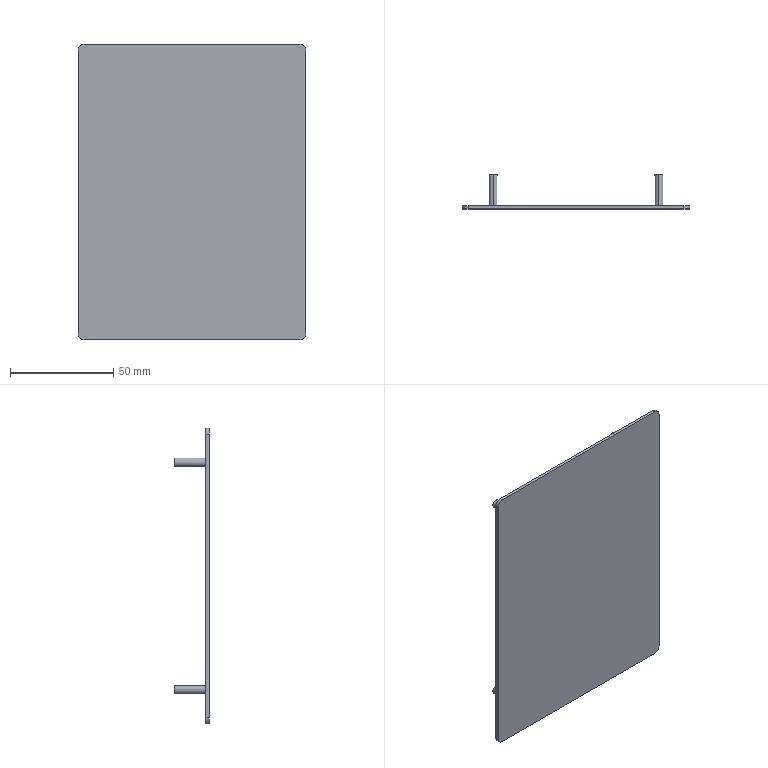Part | SolidWorks | features Extrusion 1, Fillet 1, ICE 1 | 1 solid | 22 faces | box 110 x 16.5 x 143 mm | volume 24337 mm3 | cylinder 12 | plane 10 | commonest cylinder face diameters 4 x8 6 x4
STEP:
#1=CARTESIAN_POINT('',(95.,16.5,-124.5));
#2=VERTEX_POINT('',#1);
#3=CARTESIAN_POINT('',(95.,16.5,-128.5));
#4=VERTEX_POINT('',#3);
#5=CARTESIAN_POINT('',(95.,16.5,-126.5));
#6=DIRECTION('',(0.,1.,0.));
#7=DIRECTION('',(0.,0.,-1.));
#8=AXIS2_PLACEMENT_3D('',#5,#6,#7);
#9=CIRCLE('',#8,2.);
#10=EDGE_CURVE('',#2,#4,#9,.T.);
#11=ORIENTED_EDGE('',*,*,#10,.F.);
#12=CARTESIAN_POINT('',(95.,1.5,-124.5));
#13=VERTEX_POINT('',#12);
#14=CARTESIAN_POINT('',(95.,16.5,-124.5));
#15=DIRECTION('',(0.,-1.,0.));
#16=VECTOR('',#15,1000.);
#17=LINE('',#14,#16);
#18=EDGE_CURVE('',#2,#13,#17,.T.);
#19=ORIENTED_EDGE('',*,*,#18,.T.);
#20=CARTESIAN_POINT('',(95.,1.5,-128.5));
#21=VERTEX_POINT('',#20);
#22=CARTESIAN_POINT('',(95.,1.5,-126.5));
#23=DIRECTION('',(0.,1.,0.));
#24=DIRECTION('',(0.,0.,-1.));
#25=AXIS2_PLACEMENT_3D('',#22,#23,#24);
#26=CIRCLE('',#25,2.);
#27=EDGE_CURVE('',#13,#21,#26,.T.);
#28=ORIENTED_EDGE('',*,*,#27,.T.);
#29=CARTESIAN_POINT('',(95.,16.5,-128.5));
#30=DIRECTION('',(0.,-1.,0.));
#31=VECTOR('',#30,1000.);
#32=LINE('',#29,#31);
#33=EDGE_CURVE('',#4,#21,#32,.T.);
#34=ORIENTED_EDGE('',*,*,#33,.F.);
#35=EDGE_LOOP('',(#11,#19,#28,#34));
#36=FACE_OUTER_BOUND('',#35,.T.);
#37=CARTESIAN_POINT('',(95.,16.5,-126.5));
#38=DIRECTION('',(0.,-1.,0.));
#39=DIRECTION('',(0.,0.,-1.));
#40=AXIS2_PLACEMENT_3D('',#37,#38,#39);
#41=CYLINDRICAL_SURFACE('',#40,2.);
#42=ADVANCED_FACE('',(#36),#41,.T.);
#43=CARTESIAN_POINT('',(95.,16.5,-14.5));
#44=VERTEX_POINT('',#43);
#45=CARTESIAN_POINT('',(95.,16.5,-18.5));
#46=VERTEX_POINT('',#45);
#47=CARTESIAN_POINT('',(95.,16.5,-16.5));
#48=DIRECTION('',(0.,1.,0.));
#49=DIRECTION('',(0.,0.,-1.));
#50=AXIS2_PLACEMENT_3D('',#47,#48,#49);
#51=CIRCLE('',#50,2.);
#52=EDGE_CURVE('',#44,#46,#51,.T.);
#53=ORIENTED_EDGE('',*,*,#52,.F.);
#54=CARTESIAN_POINT('',(95.,1.5,-14.5));
#55=VERTEX_POINT('',#54);
#56=CARTESIAN_POINT('',(95.,16.5,-14.5));
#57=DIRECTION('',(0.,-1.,0.));
#58=VECTOR('',#57,1000.);
#59=LINE('',#56,#58);
#60=EDGE_CURVE('',#44,#55,#59,.T.);
#61=ORIENTED_EDGE('',*,*,#60,.T.);
#62=CARTESIAN_POINT('',(95.,1.5,-18.5));
#63=VERTEX_POINT('',#62);
#64=CARTESIAN_POINT('',(95.,1.5,-16.5));
#65=DIRECTION('',(0.,1.,0.));
#66=DIRECTION('',(0.,0.,-1.));
#67=AXIS2_PLACEMENT_3D('',#64,#65,#66);
#68=CIRCLE('',#67,2.);
#69=EDGE_CURVE('',#55,#63,#68,.T.);
#70=ORIENTED_EDGE('',*,*,#69,.T.);
#71=CARTESIAN_POINT('',(95.,16.5,-18.5));
#72=DIRECTION('',(0.,-1.,0.));
#73=VECTOR('',#72,1000.);
#74=LINE('',#71,#73);
#75=EDGE_CURVE('',#46,#63,#74,.T.);
#76=ORIENTED_EDGE('',*,*,#75,.F.);
#77=EDGE_LOOP('',(#53,#61,#70,#76));
#78=FACE_OUTER_BOUND('',#77,.T.);
#79=CARTESIAN_POINT('',(95.,16.5,-16.5));
#80=DIRECTION('',(0.,-1.,0.));
#81=DIRECTION('',(0.,0.,-1.));
#82=AXIS2_PLACEMENT_3D('',#79,#80,#81);
#83=CYLINDRICAL_SURFACE('',#82,2.);
#84=ADVANCED_FACE('',(#78),#83,.T.);
#85=CARTESIAN_POINT('',(15.,16.5,-14.5));
#86=VERTEX_POINT('',#85);
#87=CARTESIAN_POINT('',(15.,16.5,-18.5));
#88=VERTEX_POINT('',#87);
#89=CARTESIAN_POINT('',(15.,16.5,-16.5));
#90=DIRECTION('',(0.,1.,0.));
#91=DIRECTION('',(0.,0.,1.));
#92=AXIS2_PLACEMENT_3D('',#89,#90,#91);
#93=CIRCLE('',#92,2.);
#94=EDGE_CURVE('',#86,#88,#93,.T.);
#95=ORIENTED_EDGE('',*,*,#94,.F.);
#96=CARTESIAN_POINT('',(15.,1.5,-14.5));
#97=VERTEX_POINT('',#96);
#98=CARTESIAN_POINT('',(15.,16.5,-14.5));
#99=DIRECTION('',(0.,-1.,0.));
#100=VECTOR('',#99,1000.);
#101=LINE('',#98,#100);
#102=EDGE_CURVE('',#86,#97,#101,.T.);
#103=ORIENTED_EDGE('',*,*,#102,.T.);
#104=CARTESIAN_POINT('',(15.,1.5,-18.5));
#105=VERTEX_POINT('',#104);
#106=CARTESIAN_POINT('',(15.,1.5,-16.5));
#107=DIRECTION('',(0.,1.,0.));
#108=DIRECTION('',(0.,0.,-1.));
#109=AXIS2_PLACEMENT_3D('',#106,#107,#108);
#110=CIRCLE('',#109,2.);
#111=EDGE_CURVE('',#97,#105,#110,.T.);
#112=ORIENTED_EDGE('',*,*,#111,.T.);
#113=CARTESIAN_POINT('',(15.,16.5,-18.5));
#114=DIRECTION('',(0.,-1.,0.));
#115=VECTOR('',#114,1000.);
#116=LINE('',#113,#115);
#117=EDGE_CURVE('',#88,#105,#116,.T.);
#118=ORIENTED_EDGE('',*,*,#117,.F.);
#119=EDGE_LOOP('',(#95,#103,#112,#118));
#120=FACE_OUTER_BOUND('',#119,.T.);
#121=CARTESIAN_POINT('',(15.,16.5,-16.5));
#122=DIRECTION('',(0.,-1.,0.));
#123=DIRECTION('',(0.,0.,-1.));
#124=AXIS2_PLACEMENT_3D('',#121,#122,#123);
#125=CYLINDRICAL_SURFACE('',#124,2.);
#126=ADVANCED_FACE('',(#120),#125,.T.);
#127=CARTESIAN_POINT('',(15.,16.5,-124.5));
#128=VERTEX_POINT('',#127);
#129=CARTESIAN_POINT('',(15.,16.5,-128.5));
#130=VERTEX_POINT('',#129);
#131=CARTESIAN_POINT('',(15.,16.5,-126.5));
#132=DIRECTION('',(0.,1.,0.));
#133=DIRECTION('',(0.,0.,1.));
#134=AXIS2_PLACEMENT_3D('',#131,#132,#133);
#135=CIRCLE('',#134,2.);
#136=EDGE_CURVE('',#128,#130,#135,.T.);
#137=ORIENTED_EDGE('',*,*,#136,.F.);
#138=CARTESIAN_POINT('',(15.,1.5,-124.5));
#139=VERTEX_POINT('',#138);
#140=CARTESIAN_POINT('',(15.,16.5,-124.5));
#141=DIRECTION('',(0.,-1.,0.));
#142=VECTOR('',#141,1000.);
#143=LINE('',#140,#142);
#144=EDGE_CURVE('',#128,#139,#143,.T.);
#145=ORIENTED_EDGE('',*,*,#144,.T.);
#146=CARTESIAN_POINT('',(15.,1.5,-128.5));
#147=VERTEX_POINT('',#146);
#148=CARTESIAN_POINT('',(15.,1.5,-126.5));
#149=DIRECTION('',(0.,1.,0.));
#150=DIRECTION('',(0.,0.,-1.));
#151=AXIS2_PLACEMENT_3D('',#148,#149,#150);
#152=CIRCLE('',#151,2.);
#153=EDGE_CURVE('',#139,#147,#152,.T.);
#154=ORIENTED_EDGE('',*,*,#153,.T.);
#155=CARTESIAN_POINT('',(15.,16.5,-128.5));
#156=DIRECTION('',(0.,-1.,0.));
#157=VECTOR('',#156,1000.);
#158=LINE('',#155,#157);
#159=EDGE_CURVE('',#130,#147,#158,.T.);
#160=ORIENTED_EDGE('',*,*,#159,.F.);
#161=EDGE_LOOP('',(#137,#145,#154,#160));
#162=FACE_OUTER_BOUND('',#161,.T.);
#163=CARTESIAN_POINT('',(15.,16.5,-126.5));
#164=DIRECTION('',(0.,-1.,0.));
#165=DIRECTION('',(0.,0.,-1.));
#166=AXIS2_PLACEMENT_3D('',#163,#164,#165);
#167=CYLINDRICAL_SURFACE('',#166,2.);
#168=ADVANCED_FACE('',(#162),#167,.T.);
#169=CARTESIAN_POINT('',(0.,1.5,-140.));
#170=VERTEX_POINT('',#169);
#171=CARTESIAN_POINT('',(0.,1.5,-3.));
#172=VERTEX_POINT('',#171);
#173=CARTESIAN_POINT('',(0.,1.5,0.));
#174=DIRECTION('',(0.,0.,1.));
#175=VECTOR('',#174,1000.);
#176=LINE('',#173,#175);
#177=EDGE_CURVE('',#170,#172,#176,.T.);
#178=ORIENTED_EDGE('',*,*,#177,.F.);
#179=CARTESIAN_POINT('',(0.,0.,-140.));
#180=VERTEX_POINT('',#179);
#181=CARTESIAN_POINT('',(0.,1.5,-140.));
#182=DIRECTION('',(0.,-1.,0.));
#183=VECTOR('',#182,1000.);
#184=LINE('',#181,#183);
#185=EDGE_CURVE('',#170,#180,#184,.T.);
#186=ORIENTED_EDGE('',*,*,#185,.T.);
#187=CARTESIAN_POINT('',(0.,0.,-3.));
#188=VERTEX_POINT('',#187);
#189=CARTESIAN_POINT('',(0.,0.,0.));
#190=DIRECTION('',(0.,0.,1.));
#191=VECTOR('',#190,1000.);
#192=LINE('',#189,#191);
#193=EDGE_CURVE('',#180,#188,#192,.T.);
#194=ORIENTED_EDGE('',*,*,#193,.T.);
#195=CARTESIAN_POINT('',(0.,1.5,-3.));
#196=DIRECTION('',(0.,1.,0.));
#197=VECTOR('',#196,1000.);
#198=LINE('',#195,#197);
#199=EDGE_CURVE('',#188,#172,#198,.T.);
#200=ORIENTED_EDGE('',*,*,#199,.T.);
#201=EDGE_LOOP('',(#178,#186,#194,#200));
#202=FACE_OUTER_BOUND('',#201,.T.);
#203=CARTESIAN_POINT('',(0.,1.5,0.));
#204=DIRECTION('',(1.,0.,0.));
#205=DIRECTION('',(0.,0.,-1.));
#206=AXIS2_PLACEMENT_3D('',#203,#204,#205);
#207=PLANE('',#206);
#208=ADVANCED_FACE('',(#202),#207,.F.);
#209=CARTESIAN_POINT('',(3.,1.5,0.));
#210=VERTEX_POINT('',#209);
#211=CARTESIAN_POINT('',(107.,1.5,0.));
#212=VERTEX_POINT('',#211);
#213=CARTESIAN_POINT('',(0.,1.5,0.));
#214=DIRECTION('',(1.,0.,0.));
#215=VECTOR('',#214,1000.);
#216=LINE('',#213,#215);
#217=EDGE_CURVE('',#210,#212,#216,.T.);
#218=ORIENTED_EDGE('',*,*,#217,.F.);
#219=CARTESIAN_POINT('',(3.,0.,0.));
#220=VERTEX_POINT('',#219);
#221=CARTESIAN_POINT('',(3.,1.5,0.));
#222=DIRECTION('',(0.,-1.,0.));
#223=VECTOR('',#222,1000.);
#224=LINE('',#221,#223);
#225=EDGE_CURVE('',#210,#220,#224,.T.);
#226=ORIENTED_EDGE('',*,*,#225,.T.);
#227=CARTESIAN_POINT('',(107.,0.,0.));
#228=VERTEX_POINT('',#227);
#229=CARTESIAN_POINT('',(0.,0.,0.));
#230=DIRECTION('',(1.,0.,0.));
#231=VECTOR('',#230,1000.);
#232=LINE('',#229,#231);
#233=EDGE_CURVE('',#220,#228,#232,.T.);
#234=ORIENTED_EDGE('',*,*,#233,.T.);
#235=CARTESIAN_POINT('',(107.,1.5,0.));
#236=DIRECTION('',(0.,1.,0.));
#237=VECTOR('',#236,1000.);
#238=LINE('',#235,#237);
#239=EDGE_CURVE('',#228,#212,#238,.T.);
#240=ORIENTED_EDGE('',*,*,#239,.T.);
#241=EDGE_LOOP('',(#218,#226,#234,#240));
#242=FACE_OUTER_BOUND('',#241,.T.);
#243=CARTESIAN_POINT('',(0.,1.5,0.));
#244=DIRECTION('',(0.,0.,-1.));
#245=DIRECTION('',(-1.,0.,0.));
#246=AXIS2_PLACEMENT_3D('',#243,#244,#245);
#247=PLANE('',#246);
#248=ADVANCED_FACE('',(#242),#247,.F.);
#249=CARTESIAN_POINT('',(110.,0.,-3.));
#250=VERTEX_POINT('',#249);
#251=CARTESIAN_POINT('',(110.,0.,-140.));
#252=VERTEX_POINT('',#251);
#253=CARTESIAN_POINT('',(110.,0.,0.));
#254=DIRECTION('',(0.,0.,-1.));
#255=VECTOR('',#254,1000.);
#256=LINE('',#253,#255);
#257=EDGE_CURVE('',#250,#252,#256,.T.);
#258=ORIENTED_EDGE('',*,*,#257,.T.);
#259=CARTESIAN_POINT('',(110.,1.5,-140.));
#260=VERTEX_POINT('',#259);
#261=CARTESIAN_POINT('',(110.,1.5,-140.));
#262=DIRECTION('',(0.,1.,0.));
#263=VECTOR('',#262,1000.);
#264=LINE('',#261,#263);
#265=EDGE_CURVE('',#252,#260,#264,.T.);
#266=ORIENTED_EDGE('',*,*,#265,.T.);
#267=CARTESIAN_POINT('',(110.,1.5,-3.));
#268=VERTEX_POINT('',#267);
#269=CARTESIAN_POINT('',(110.,1.5,0.));
#270=DIRECTION('',(0.,0.,-1.));
#271=VECTOR('',#270,1000.);
#272=LINE('',#269,#271);
#273=EDGE_CURVE('',#268,#260,#272,.T.);
#274=ORIENTED_EDGE('',*,*,#273,.F.);
#275=CARTESIAN_POINT('',(110.,1.5,-3.));
#276=DIRECTION('',(0.,-1.,0.));
#277=VECTOR('',#276,1000.);
#278=LINE('',#275,#277);
#279=EDGE_CURVE('',#268,#250,#278,.T.);
#280=ORIENTED_EDGE('',*,*,#279,.T.);
#281=EDGE_LOOP('',(#258,#266,#274,#280));
#282=FACE_OUTER_BOUND('',#281,.T.);
#283=CARTESIAN_POINT('',(110.,1.5,0.));
#284=DIRECTION('',(-1.,0.,0.));
#285=DIRECTION('',(0.,0.,1.));
#286=AXIS2_PLACEMENT_3D('',#283,#284,#285);
#287=PLANE('',#286);
#288=ADVANCED_FACE('',(#282),#287,.F.);
#289=CARTESIAN_POINT('',(107.,0.,-143.));
#290=VERTEX_POINT('',#289);
#291=CARTESIAN_POINT('',(3.,0.,-143.));
#292=VERTEX_POINT('',#291);
#293=CARTESIAN_POINT('',(0.,0.,-143.));
#294=DIRECTION('',(-1.,0.,0.));
#295=VECTOR('',#294,1000.);
#296=LINE('',#293,#295);
#297=EDGE_CURVE('',#290,#292,#296,.T.);
#298=ORIENTED_EDGE('',*,*,#297,.T.);
#299=CARTESIAN_POINT('',(3.,1.5,-143.));
#300=VERTEX_POINT('',#299);
#301=CARTESIAN_POINT('',(3.,1.5,-143.));
#302=DIRECTION('',(0.,1.,0.));
#303=VECTOR('',#302,1000.);
#304=LINE('',#301,#303);
#305=EDGE_CURVE('',#292,#300,#304,.T.);
#306=ORIENTED_EDGE('',*,*,#305,.T.);
#307=CARTESIAN_POINT('',(107.,1.5,-143.));
#308=VERTEX_POINT('',#307);
#309=CARTESIAN_POINT('',(0.,1.5,-143.));
#310=DIRECTION('',(-1.,0.,0.));
#311=VECTOR('',#310,1000.);
#312=LINE('',#309,#311);
#313=EDGE_CURVE('',#308,#300,#312,.T.);
#314=ORIENTED_EDGE('',*,*,#313,.F.);
#315=CARTESIAN_POINT('',(107.,1.5,-143.));
#316=DIRECTION('',(0.,-1.,0.));
#317=VECTOR('',#316,1000.);
#318=LINE('',#315,#317);
#319=EDGE_CURVE('',#308,#290,#318,.T.);
#320=ORIENTED_EDGE('',*,*,#319,.T.);
#321=EDGE_LOOP('',(#298,#306,#314,#320));
#322=FACE_OUTER_BOUND('',#321,.T.);
#323=CARTESIAN_POINT('',(0.,1.5,-143.));
#324=DIRECTION('',(0.,0.,1.));
#325=DIRECTION('',(1.,0.,0.));
#326=AXIS2_PLACEMENT_3D('',#323,#324,#325);
#327=PLANE('',#326);
#328=ADVANCED_FACE('',(#322),#327,.F.);
#329=CARTESIAN_POINT('',(95.,1.5,-126.5));
#330=DIRECTION('',(0.,1.,0.));
#331=DIRECTION('',(0.,0.,-1.));
#332=AXIS2_PLACEMENT_3D('',#329,#330,#331);
#333=CIRCLE('',#332,2.);
#334=EDGE_CURVE('',#21,#13,#333,.T.);
#335=ORIENTED_EDGE('',*,*,#334,.F.);
#336=ORIENTED_EDGE('',*,*,#27,.F.);
#337=EDGE_LOOP('',(#335,#336));
#338=FACE_BOUND('',#337,.T.);
#339=CARTESIAN_POINT('',(95.,1.5,-16.5));
#340=DIRECTION('',(0.,1.,0.));
#341=DIRECTION('',(0.,0.,-1.));
#342=AXIS2_PLACEMENT_3D('',#339,#340,#341);
#343=CIRCLE('',#342,2.);
#344=EDGE_CURVE('',#63,#55,#343,.T.);
#345=ORIENTED_EDGE('',*,*,#344,.F.);
#346=ORIENTED_EDGE('',*,*,#69,.F.);
#347=EDGE_LOOP('',(#345,#346));
#348=FACE_BOUND('',#347,.T.);
#349=CARTESIAN_POINT('',(15.,1.5,-16.5));
#350=DIRECTION('',(0.,1.,0.));
#351=DIRECTION('',(0.,0.,-1.));
#352=AXIS2_PLACEMENT_3D('',#349,#350,#351);
#353=CIRCLE('',#352,2.);
#354=EDGE_CURVE('',#105,#97,#353,.T.);
#355=ORIENTED_EDGE('',*,*,#354,.F.);
#356=ORIENTED_EDGE('',*,*,#111,.F.);
#357=EDGE_LOOP('',(#355,#356));
#358=FACE_BOUND('',#357,.T.);
#359=CARTESIAN_POINT('',(15.,1.5,-126.5));
#360=DIRECTION('',(0.,1.,0.));
#361=DIRECTION('',(0.,0.,-1.));
#362=AXIS2_PLACEMENT_3D('',#359,#360,#361);
#363=CIRCLE('',#362,2.);
#364=EDGE_CURVE('',#147,#139,#363,.T.);
#365=ORIENTED_EDGE('',*,*,#364,.F.);
#366=ORIENTED_EDGE('',*,*,#153,.F.);
#367=EDGE_LOOP('',(#365,#366));
#368=FACE_BOUND('',#367,.T.);
#369=ORIENTED_EDGE('',*,*,#313,.T.);
#370=CARTESIAN_POINT('',(3.,1.5,-140.));
#371=DIRECTION('',(0.,1.,0.));
#372=DIRECTION('',(0.,0.,-1.));
#373=AXIS2_PLACEMENT_3D('',#370,#371,#372);
#374=CIRCLE('',#373,3.);
#375=EDGE_CURVE('',#300,#170,#374,.T.);
#376=ORIENTED_EDGE('',*,*,#375,.T.);
#377=ORIENTED_EDGE('',*,*,#177,.T.);
#378=CARTESIAN_POINT('',(3.,1.5,-3.));
#379=DIRECTION('',(0.,1.,0.));
#380=DIRECTION('',(0.,0.,-1.));
#381=AXIS2_PLACEMENT_3D('',#378,#379,#380);
#382=CIRCLE('',#381,3.);
#383=EDGE_CURVE('',#172,#210,#382,.T.);
#384=ORIENTED_EDGE('',*,*,#383,.T.);
#385=ORIENTED_EDGE('',*,*,#217,.T.);
#386=CARTESIAN_POINT('',(107.,1.5,-3.));
#387=DIRECTION('',(0.,1.,0.));
#388=DIRECTION('',(0.,0.,-1.));
#389=AXIS2_PLACEMENT_3D('',#386,#387,#388);
#390=CIRCLE('',#389,3.);
#391=EDGE_CURVE('',#212,#268,#390,.T.);
#392=ORIENTED_EDGE('',*,*,#391,.T.);
#393=ORIENTED_EDGE('',*,*,#273,.T.);
#394=CARTESIAN_POINT('',(107.,1.5,-140.));
#395=DIRECTION('',(0.,1.,0.));
#396=DIRECTION('',(0.,0.,-1.));
#397=AXIS2_PLACEMENT_3D('',#394,#395,#396);
#398=CIRCLE('',#397,3.);
#399=EDGE_CURVE('',#260,#308,#398,.T.);
#400=ORIENTED_EDGE('',*,*,#399,.T.);
#401=EDGE_LOOP('',(#369,#376,#377,#384,#385,#392,#393,#400));
#402=FACE_OUTER_BOUND('',#401,.T.);
#403=CARTESIAN_POINT('',(0.,1.5,0.));
#404=DIRECTION('',(0.,-1.,0.));
#405=DIRECTION('',(0.,0.,-1.));
#406=AXIS2_PLACEMENT_3D('',#403,#404,#405);
#407=PLANE('',#406);
#408=ADVANCED_FACE('',(#338,#348,#358,#368,#402),#407,.F.);
#409=ORIENTED_EDGE('',*,*,#193,.F.);
#410=CARTESIAN_POINT('',(3.,0.,-140.));
#411=DIRECTION('',(0.,-1.,0.));
#412=DIRECTION('',(0.,0.,-1.));
#413=AXIS2_PLACEMENT_3D('',#410,#411,#412);
#414=CIRCLE('',#413,3.);
#415=EDGE_CURVE('',#180,#292,#414,.T.);
#416=ORIENTED_EDGE('',*,*,#415,.T.);
#417=ORIENTED_EDGE('',*,*,#297,.F.);
#418=CARTESIAN_POINT('',(107.,0.,-140.));
#419=DIRECTION('',(0.,-1.,0.));
#420=DIRECTION('',(0.,0.,-1.));
#421=AXIS2_PLACEMENT_3D('',#418,#419,#420);
#422=CIRCLE('',#421,3.);
#423=EDGE_CURVE('',#290,#252,#422,.T.);
#424=ORIENTED_EDGE('',*,*,#423,.T.);
#425=ORIENTED_EDGE('',*,*,#257,.F.);
#426=CARTESIAN_POINT('',(107.,0.,-3.));
#427=DIRECTION('',(0.,-1.,0.));
#428=DIRECTION('',(0.,0.,-1.));
#429=AXIS2_PLACEMENT_3D('',#426,#427,#428);
#430=CIRCLE('',#429,3.);
#431=EDGE_CURVE('',#250,#228,#430,.T.);
#432=ORIENTED_EDGE('',*,*,#431,.T.);
#433=ORIENTED_EDGE('',*,*,#233,.F.);
#434=CARTESIAN_POINT('',(3.,0.,-3.));
#435=DIRECTION('',(0.,-1.,0.));
#436=DIRECTION('',(0.,0.,-1.));
#437=AXIS2_PLACEMENT_3D('',#434,#435,#436);
#438=CIRCLE('',#437,3.);
#439=EDGE_CURVE('',#220,#188,#438,.T.);
#440=ORIENTED_EDGE('',*,*,#439,.T.);
#441=EDGE_LOOP('',(#409,#416,#417,#424,#425,#432,#433,#440));
#442=FACE_OUTER_BOUND('',#441,.T.);
#443=CARTESIAN_POINT('',(0.,0.,0.));
#444=DIRECTION('',(0.,-1.,0.));
#445=DIRECTION('',(0.,0.,-1.));
#446=AXIS2_PLACEMENT_3D('',#443,#444,#445);
#447=PLANE('',#446);
#448=ADVANCED_FACE('',(#442),#447,.T.);
#449=ORIENTED_EDGE('',*,*,#375,.F.);
#450=ORIENTED_EDGE('',*,*,#305,.F.);
#451=ORIENTED_EDGE('',*,*,#415,.F.);
#452=ORIENTED_EDGE('',*,*,#185,.F.);
#453=EDGE_LOOP('',(#449,#450,#451,#452));
#454=FACE_OUTER_BOUND('',#453,.T.);
#455=CARTESIAN_POINT('',(3.,1.5,-140.));
#456=DIRECTION('',(0.,-1.,0.));
#457=DIRECTION('',(0.,0.,-1.));
#458=AXIS2_PLACEMENT_3D('',#455,#456,#457);
#459=CYLINDRICAL_SURFACE('',#458,3.);
#460=ADVANCED_FACE('',(#454),#459,.T.);
#461=ORIENTED_EDGE('',*,*,#383,.F.);
#462=ORIENTED_EDGE('',*,*,#199,.F.);
#463=ORIENTED_EDGE('',*,*,#439,.F.);
#464=ORIENTED_EDGE('',*,*,#225,.F.);
#465=EDGE_LOOP('',(#461,#462,#463,#464));
#466=FACE_OUTER_BOUND('',#465,.T.);
#467=CARTESIAN_POINT('',(3.,1.5,-3.));
#468=DIRECTION('',(0.,-1.,0.));
#469=DIRECTION('',(0.,0.,-1.));
#470=AXIS2_PLACEMENT_3D('',#467,#468,#469);
#471=CYLINDRICAL_SURFACE('',#470,3.);
#472=ADVANCED_FACE('',(#466),#471,.T.);
#473=ORIENTED_EDGE('',*,*,#399,.F.);
#474=ORIENTED_EDGE('',*,*,#265,.F.);
#475=ORIENTED_EDGE('',*,*,#423,.F.);
#476=ORIENTED_EDGE('',*,*,#319,.F.);
#477=EDGE_LOOP('',(#473,#474,#475,#476));
#478=FACE_OUTER_BOUND('',#477,.T.);
#479=CARTESIAN_POINT('',(107.,1.5,-140.));
#480=DIRECTION('',(0.,-1.,0.));
#481=DIRECTION('',(0.,0.,-1.));
#482=AXIS2_PLACEMENT_3D('',#479,#480,#481);
#483=CYLINDRICAL_SURFACE('',#482,3.);
#484=ADVANCED_FACE('',(#478),#483,.T.);
#485=ORIENTED_EDGE('',*,*,#391,.F.);
#486=ORIENTED_EDGE('',*,*,#239,.F.);
#487=ORIENTED_EDGE('',*,*,#431,.F.);
#488=ORIENTED_EDGE('',*,*,#279,.F.);
#489=EDGE_LOOP('',(#485,#486,#487,#488));
#490=FACE_OUTER_BOUND('',#489,.T.);
#491=CARTESIAN_POINT('',(107.,1.5,-3.));
#492=DIRECTION('',(0.,-1.,0.));
#493=DIRECTION('',(0.,0.,-1.));
#494=AXIS2_PLACEMENT_3D('',#491,#492,#493);
#495=CYLINDRICAL_SURFACE('',#494,3.);
#496=ADVANCED_FACE('',(#490),#495,.T.);
#497=ORIENTED_EDGE('',*,*,#144,.F.);
#498=CARTESIAN_POINT('',(15.,16.5,-126.5));
#499=DIRECTION('',(0.,1.,0.));
#500=DIRECTION('',(0.,0.,1.));
#501=AXIS2_PLACEMENT_3D('',#498,#499,#500);
#502=CIRCLE('',#501,2.);
#503=EDGE_CURVE('',#130,#128,#502,.T.);
#504=ORIENTED_EDGE('',*,*,#503,.F.);
#505=ORIENTED_EDGE('',*,*,#159,.T.);
#506=ORIENTED_EDGE('',*,*,#364,.T.);
#507=EDGE_LOOP('',(#497,#504,#505,#506));
#508=FACE_OUTER_BOUND('',#507,.T.);
#509=CARTESIAN_POINT('',(15.,16.5,-126.5));
#510=DIRECTION('',(0.,-1.,0.));
#511=DIRECTION('',(0.,0.,-1.));
#512=AXIS2_PLACEMENT_3D('',#509,#510,#511);
#513=CYLINDRICAL_SURFACE('',#512,2.);
#514=ADVANCED_FACE('',(#508),#513,.T.);
#515=ORIENTED_EDGE('',*,*,#503,.T.);
#516=ORIENTED_EDGE('',*,*,#136,.T.);
#517=EDGE_LOOP('',(#515,#516));
#518=FACE_OUTER_BOUND('',#517,.T.);
#519=CARTESIAN_POINT('',(15.,16.5,-126.5));
#520=DIRECTION('',(0.,1.,0.));
#521=DIRECTION('',(0.,0.,1.));
#522=AXIS2_PLACEMENT_3D('',#519,#520,#521);
#523=PLANE('',#522);
#524=ADVANCED_FACE('',(#518),#523,.T.);
#525=ORIENTED_EDGE('',*,*,#102,.F.);
#526=CARTESIAN_POINT('',(15.,16.5,-16.5));
#527=DIRECTION('',(0.,1.,0.));
#528=DIRECTION('',(0.,0.,1.));
#529=AXIS2_PLACEMENT_3D('',#526,#527,#528);
#530=CIRCLE('',#529,2.);
#531=EDGE_CURVE('',#88,#86,#530,.T.);
#532=ORIENTED_EDGE('',*,*,#531,.F.);
#533=ORIENTED_EDGE('',*,*,#117,.T.);
#534=ORIENTED_EDGE('',*,*,#354,.T.);
#535=EDGE_LOOP('',(#525,#532,#533,#534));
#536=FACE_OUTER_BOUND('',#535,.T.);
#537=CARTESIAN_POINT('',(15.,16.5,-16.5));
#538=DIRECTION('',(0.,-1.,0.));
#539=DIRECTION('',(0.,0.,-1.));
#540=AXIS2_PLACEMENT_3D('',#537,#538,#539);
#541=CYLINDRICAL_SURFACE('',#540,2.);
#542=ADVANCED_FACE('',(#536),#541,.T.);
#543=ORIENTED_EDGE('',*,*,#531,.T.);
#544=ORIENTED_EDGE('',*,*,#94,.T.);
#545=EDGE_LOOP('',(#543,#544));
#546=FACE_OUTER_BOUND('',#545,.T.);
#547=CARTESIAN_POINT('',(15.,16.5,-16.5));
#548=DIRECTION('',(0.,1.,0.));
#549=DIRECTION('',(0.,0.,1.));
#550=AXIS2_PLACEMENT_3D('',#547,#548,#549);
#551=PLANE('',#550);
#552=ADVANCED_FACE('',(#546),#551,.T.);
#553=ORIENTED_EDGE('',*,*,#60,.F.);
#554=CARTESIAN_POINT('',(95.,16.5,-16.5));
#555=DIRECTION('',(0.,1.,0.));
#556=DIRECTION('',(0.,0.,-1.));
#557=AXIS2_PLACEMENT_3D('',#554,#555,#556);
#558=CIRCLE('',#557,2.);
#559=EDGE_CURVE('',#46,#44,#558,.T.);
#560=ORIENTED_EDGE('',*,*,#559,.F.);
#561=ORIENTED_EDGE('',*,*,#75,.T.);
#562=ORIENTED_EDGE('',*,*,#344,.T.);
#563=EDGE_LOOP('',(#553,#560,#561,#562));
#564=FACE_OUTER_BOUND('',#563,.T.);
#565=CARTESIAN_POINT('',(95.,16.5,-16.5));
#566=DIRECTION('',(0.,-1.,0.));
#567=DIRECTION('',(0.,0.,-1.));
#568=AXIS2_PLACEMENT_3D('',#565,#566,#567);
#569=CYLINDRICAL_SURFACE('',#568,2.);
#570=ADVANCED_FACE('',(#564),#569,.T.);
#571=ORIENTED_EDGE('',*,*,#559,.T.);
#572=ORIENTED_EDGE('',*,*,#52,.T.);
#573=EDGE_LOOP('',(#571,#572));
#574=FACE_OUTER_BOUND('',#573,.T.);
#575=CARTESIAN_POINT('',(95.,16.5,-16.5));
#576=DIRECTION('',(0.,-1.,0.));
#577=DIRECTION('',(0.,0.,-1.));
#578=AXIS2_PLACEMENT_3D('',#575,#576,#577);
#579=PLANE('',#578);
#580=ADVANCED_FACE('',(#574),#579,.F.);
#581=ORIENTED_EDGE('',*,*,#18,.F.);
#582=CARTESIAN_POINT('',(95.,16.5,-126.5));
#583=DIRECTION('',(0.,1.,0.));
#584=DIRECTION('',(0.,0.,-1.));
#585=AXIS2_PLACEMENT_3D('',#582,#583,#584);
#586=CIRCLE('',#585,2.);
#587=EDGE_CURVE('',#4,#2,#586,.T.);
#588=ORIENTED_EDGE('',*,*,#587,.F.);
#589=ORIENTED_EDGE('',*,*,#33,.T.);
#590=ORIENTED_EDGE('',*,*,#334,.T.);
#591=EDGE_LOOP('',(#581,#588,#589,#590));
#592=FACE_OUTER_BOUND('',#591,.T.);
#593=CARTESIAN_POINT('',(95.,16.5,-126.5));
#594=DIRECTION('',(0.,-1.,0.));
#595=DIRECTION('',(0.,0.,-1.));
#596=AXIS2_PLACEMENT_3D('',#593,#594,#595);
#597=CYLINDRICAL_SURFACE('',#596,2.);
#598=ADVANCED_FACE('',(#592),#597,.T.);
#599=ORIENTED_EDGE('',*,*,#587,.T.);
#600=ORIENTED_EDGE('',*,*,#10,.T.);
#601=EDGE_LOOP('',(#599,#600));
#602=FACE_OUTER_BOUND('',#601,.T.);
#603=CARTESIAN_POINT('',(95.,16.5,-126.5));
#604=DIRECTION('',(0.,-1.,0.));
#605=DIRECTION('',(0.,0.,-1.));
#606=AXIS2_PLACEMENT_3D('',#603,#604,#605);
#607=PLANE('',#606);
#608=ADVANCED_FACE('',(#602),#607,.F.);
#609=CLOSED_SHELL('',(#42,#84,#126,#168,#208,#248,#288,#328,#408,#448,#460,#472,#484,#496,#514,#524,#542,#552,#570,#580,#598,#608));
#610=MANIFOLD_SOLID_BREP('',#609);
#611=CARTESIAN_POINT('',(0.,0.,0.));
#612=DIRECTION('',(0.,0.,1.));
#613=DIRECTION('',(1.,0.,0.));
#614=AXIS2_PLACEMENT_3D('',#611,#612,#613);
#615=(LENGTH_UNIT()NAMED_UNIT(*)SI_UNIT(.MILLI.,.METRE.));
#616=UNCERTAINTY_MEASURE_WITH_UNIT(LENGTH_MEASURE(0.00001),#615,'','');
#617=(NAMED_UNIT(*)PLANE_ANGLE_UNIT()SI_UNIT($,.RADIAN.));
#618=(NAMED_UNIT(*)SI_UNIT($,.STERADIAN.)SOLID_ANGLE_UNIT());
#619=(GEOMETRIC_REPRESENTATION_CONTEXT(3)GLOBAL_UNCERTAINTY_ASSIGNED_CONTEXT((#616))GLOBAL_UNIT_ASSIGNED_CONTEXT((#615,#617,#618))REPRESENTATION_CONTEXT('',''));
#620=ADVANCED_BREP_SHAPE_REPRESENTATION('',(#610,#614),#619);